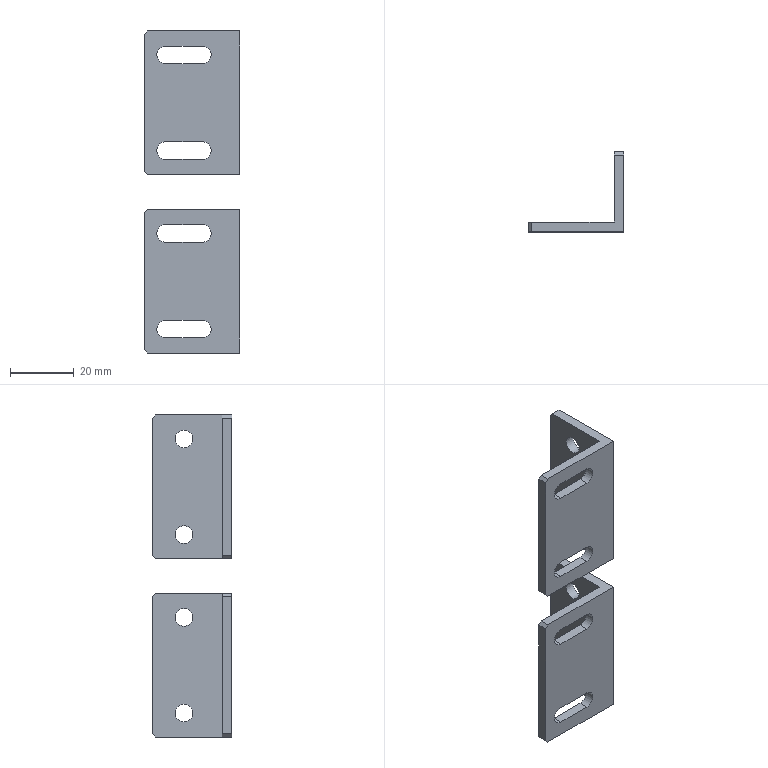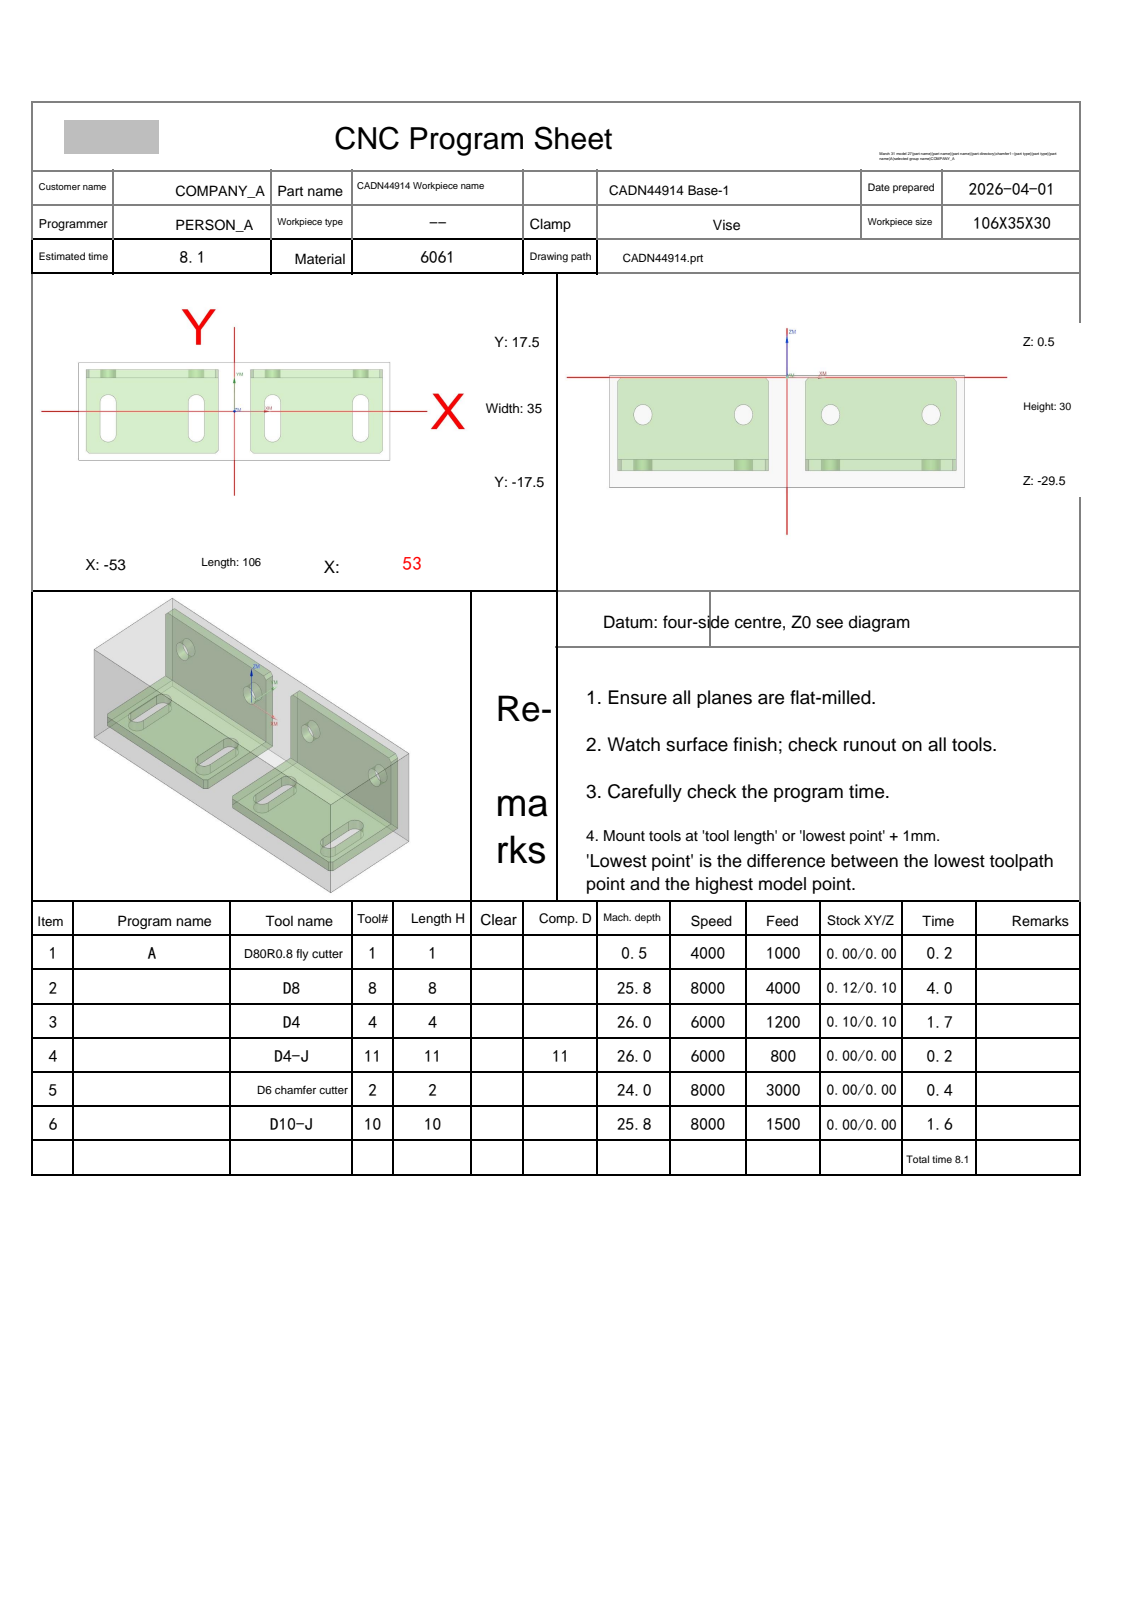NC program | NX | posted by the shop | part box 30 x 25 x 101 mm
Lines 1 to 32 of 5910:
%
O0001
(Machine time: 9.12 MIN)
(===Total Tool:6===)
(T1=D80R0.8 fly cutter D=80.  R=0.8  D-  H01 Z=0.    )
(T8=D8      D=8.   R=0.   D-  H08 Z=-25.3 )
(T4=D4      D=4.   R=0.   D-  H04 Z=-25.5 )
(T11=D4-J   D=4.   R=0.   D11 H11 Z=-25.5 )
(T2=D6 chamfer cutter   D=6.   R=0.   D-  H02 Z=-23.5 )
(T10=D10-J  D=10.  R=0.   D10 H10 Z=-25.3 )
G80 G90 G17 G49 G40
G91 G28 Z0
M01
N1 T01 M06
(D80R0.8 fly cutter  D=80. R=0.8 H=01 ce=0.00 di=0.00)
G00 G90 G54 X95.5 Y0.0 M03 S4000
G43 H01 Z20.
M08
Z2.
G01 Z0.0 F1000.
X90.5
X-90.5
X-95.5
Z2.
G00 Z20.
G91 G28 Z0.0
M05
M09
G91 G28 Z0.0
M01